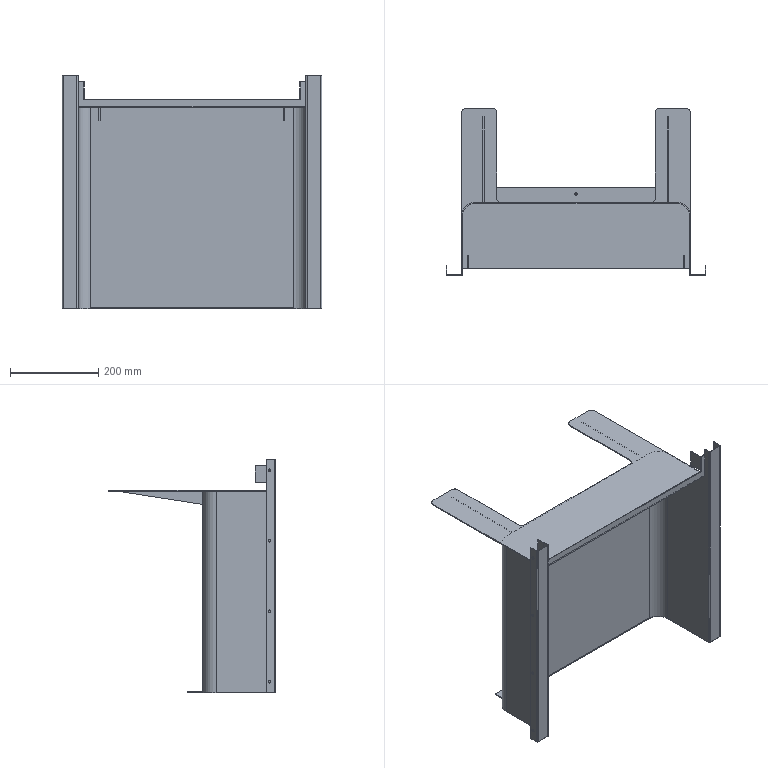Part | SolidWorks | features ICE 9, Fillet 6, HoleWzd 3, Cut 2, ExtruThin 1 | 3 solids | 100 faces | box 589 x 380 x 530 mm | volume 943074 mm3 | plane 58 | cylinder 42 | commonest cylinder face diameters 6 x26 3 x6 20 x6 57 x2 60 x2